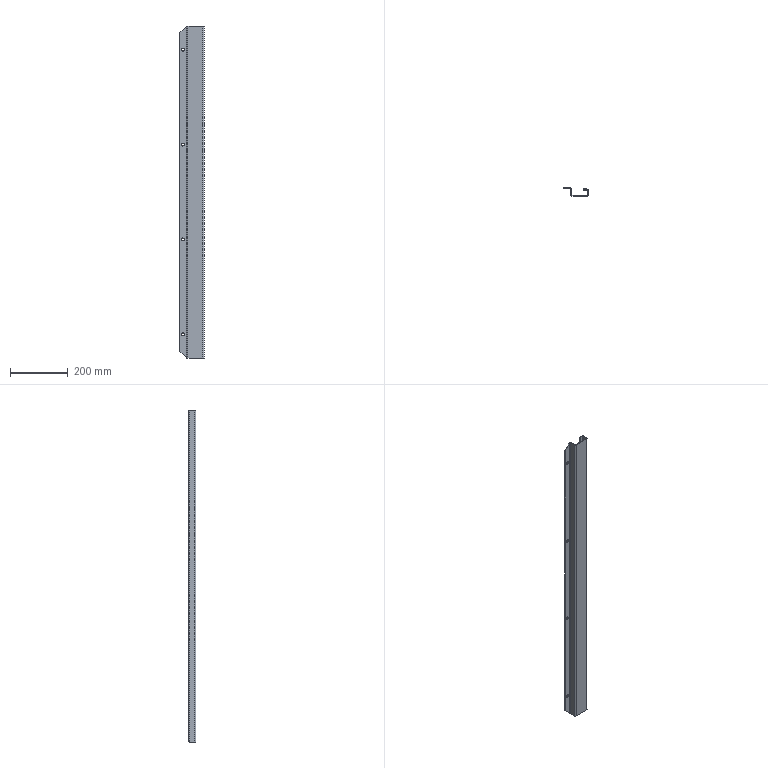Part | STEP file | 750038191 | 1 solid | 34 faces | box 84 x 27 x 1154 mm | volume 316306 mm3 | cylinder 16 | plane 16 | spline 2 | commonest cylinder face diameters 10.5 x8 4 x4 8 x4
STEP:
#1=CARTESIAN_POINT('',(-44.,27.,159.75));
#2=VERTEX_POINT('',#1);
#3=CARTESIAN_POINT('',(-44.,27.,170.25));
#4=VERTEX_POINT('',#3);
#5=CARTESIAN_POINT('',(-44.,27.,165.));
#6=DIRECTION('',(0.,1.,0.));
#7=DIRECTION('',(0.,0.,-1.));
#8=AXIS2_PLACEMENT_3D('',#5,#6,#7);
#9=CIRCLE('',#8,5.25);
#10=EDGE_CURVE('',#2,#4,#9,.T.);
#11=ORIENTED_EDGE('',*,*,#10,.T.);
#12=CARTESIAN_POINT('',(-44.,25.,170.25));
#13=VERTEX_POINT('',#12);
#14=CARTESIAN_POINT('',(-44.,1182.368,170.25));
#15=DIRECTION('',(0.,-1.,0.));
#16=VECTOR('',#15,1000.);
#17=LINE('',#14,#16);
#18=EDGE_CURVE('',#4,#13,#17,.T.);
#19=ORIENTED_EDGE('',*,*,#18,.T.);
#20=CARTESIAN_POINT('',(-44.,25.,159.75));
#21=VERTEX_POINT('',#20);
#22=CARTESIAN_POINT('',(-44.,25.,165.));
#23=DIRECTION('',(0.,1.,0.));
#24=DIRECTION('',(0.,0.,-1.));
#25=AXIS2_PLACEMENT_3D('',#22,#23,#24);
#26=CIRCLE('',#25,5.25);
#27=EDGE_CURVE('',#21,#13,#26,.T.);
#28=ORIENTED_EDGE('',*,*,#27,.F.);
#29=CARTESIAN_POINT('',(-44.,1182.368,159.75));
#30=DIRECTION('',(0.,-1.,0.));
#31=VECTOR('',#30,1000.);
#32=LINE('',#29,#31);
#33=EDGE_CURVE('',#2,#21,#32,.T.);
#34=ORIENTED_EDGE('',*,*,#33,.F.);
#35=EDGE_LOOP('',(#11,#19,#28,#34));
#36=FACE_OUTER_BOUND('',#35,.T.);
#37=CARTESIAN_POINT('',(-44.,1182.368,165.));
#38=DIRECTION('',(0.,-1.,0.));
#39=DIRECTION('',(0.,0.,-1.));
#40=AXIS2_PLACEMENT_3D('',#37,#38,#39);
#41=CYLINDRICAL_SURFACE('',#40,5.25);
#42=ADVANCED_FACE('',(#36),#41,.F.);
#43=CARTESIAN_POINT('',(-44.,27.,-500.25));
#44=VERTEX_POINT('',#43);
#45=CARTESIAN_POINT('',(-44.,27.,-489.75));
#46=VERTEX_POINT('',#45);
#47=CARTESIAN_POINT('',(-44.,27.,-495.));
#48=DIRECTION('',(0.,1.,0.));
#49=DIRECTION('',(0.,0.,-1.));
#50=AXIS2_PLACEMENT_3D('',#47,#48,#49);
#51=CIRCLE('',#50,5.25);
#52=EDGE_CURVE('',#44,#46,#51,.T.);
#53=ORIENTED_EDGE('',*,*,#52,.T.);
#54=CARTESIAN_POINT('',(-44.,25.,-489.75));
#55=VERTEX_POINT('',#54);
#56=CARTESIAN_POINT('',(-44.,1182.368,-489.75));
#57=DIRECTION('',(0.,-1.,0.));
#58=VECTOR('',#57,1000.);
#59=LINE('',#56,#58);
#60=EDGE_CURVE('',#46,#55,#59,.T.);
#61=ORIENTED_EDGE('',*,*,#60,.T.);
#62=CARTESIAN_POINT('',(-44.,25.,-500.25));
#63=VERTEX_POINT('',#62);
#64=CARTESIAN_POINT('',(-44.,25.,-495.));
#65=DIRECTION('',(0.,1.,0.));
#66=DIRECTION('',(0.,0.,-1.));
#67=AXIS2_PLACEMENT_3D('',#64,#65,#66);
#68=CIRCLE('',#67,5.25);
#69=EDGE_CURVE('',#63,#55,#68,.T.);
#70=ORIENTED_EDGE('',*,*,#69,.F.);
#71=CARTESIAN_POINT('',(-44.,1182.368,-500.25));
#72=DIRECTION('',(0.,-1.,0.));
#73=VECTOR('',#72,1000.);
#74=LINE('',#71,#73);
#75=EDGE_CURVE('',#44,#63,#74,.T.);
#76=ORIENTED_EDGE('',*,*,#75,.F.);
#77=EDGE_LOOP('',(#53,#61,#70,#76));
#78=FACE_OUTER_BOUND('',#77,.T.);
#79=CARTESIAN_POINT('',(-44.,1182.368,-495.));
#80=DIRECTION('',(0.,-1.,0.));
#81=DIRECTION('',(0.,0.,-1.));
#82=AXIS2_PLACEMENT_3D('',#79,#80,#81);
#83=CYLINDRICAL_SURFACE('',#82,5.25);
#84=ADVANCED_FACE('',(#78),#83,.F.);
#85=CARTESIAN_POINT('',(-44.,27.,-170.25));
#86=VERTEX_POINT('',#85);
#87=CARTESIAN_POINT('',(-44.,27.,-159.75));
#88=VERTEX_POINT('',#87);
#89=CARTESIAN_POINT('',(-44.,27.,-165.));
#90=DIRECTION('',(0.,1.,0.));
#91=DIRECTION('',(0.,0.,-1.));
#92=AXIS2_PLACEMENT_3D('',#89,#90,#91);
#93=CIRCLE('',#92,5.25);
#94=EDGE_CURVE('',#86,#88,#93,.T.);
#95=ORIENTED_EDGE('',*,*,#94,.T.);
#96=CARTESIAN_POINT('',(-44.,25.,-159.75));
#97=VERTEX_POINT('',#96);
#98=CARTESIAN_POINT('',(-44.,1182.368,-159.75));
#99=DIRECTION('',(0.,-1.,0.));
#100=VECTOR('',#99,1000.);
#101=LINE('',#98,#100);
#102=EDGE_CURVE('',#88,#97,#101,.T.);
#103=ORIENTED_EDGE('',*,*,#102,.T.);
#104=CARTESIAN_POINT('',(-44.,25.,-170.25));
#105=VERTEX_POINT('',#104);
#106=CARTESIAN_POINT('',(-44.,25.,-165.));
#107=DIRECTION('',(0.,1.,0.));
#108=DIRECTION('',(0.,0.,-1.));
#109=AXIS2_PLACEMENT_3D('',#106,#107,#108);
#110=CIRCLE('',#109,5.25);
#111=EDGE_CURVE('',#105,#97,#110,.T.);
#112=ORIENTED_EDGE('',*,*,#111,.F.);
#113=CARTESIAN_POINT('',(-44.,1182.368,-170.25));
#114=DIRECTION('',(0.,-1.,0.));
#115=VECTOR('',#114,1000.);
#116=LINE('',#113,#115);
#117=EDGE_CURVE('',#86,#105,#116,.T.);
#118=ORIENTED_EDGE('',*,*,#117,.F.);
#119=EDGE_LOOP('',(#95,#103,#112,#118));
#120=FACE_OUTER_BOUND('',#119,.T.);
#121=CARTESIAN_POINT('',(-44.,1182.368,-165.));
#122=DIRECTION('',(0.,-1.,0.));
#123=DIRECTION('',(0.,0.,-1.));
#124=AXIS2_PLACEMENT_3D('',#121,#122,#123);
#125=CYLINDRICAL_SURFACE('',#124,5.25);
#126=ADVANCED_FACE('',(#120),#125,.F.);
#127=CARTESIAN_POINT('',(-44.,27.,489.75));
#128=VERTEX_POINT('',#127);
#129=CARTESIAN_POINT('',(-44.,27.,500.25));
#130=VERTEX_POINT('',#129);
#131=CARTESIAN_POINT('',(-44.,27.,495.));
#132=DIRECTION('',(0.,1.,0.));
#133=DIRECTION('',(0.,0.,-1.));
#134=AXIS2_PLACEMENT_3D('',#131,#132,#133);
#135=CIRCLE('',#134,5.25);
#136=EDGE_CURVE('',#128,#130,#135,.T.);
#137=ORIENTED_EDGE('',*,*,#136,.T.);
#138=CARTESIAN_POINT('',(-44.,25.,500.25));
#139=VERTEX_POINT('',#138);
#140=CARTESIAN_POINT('',(-44.,1182.368,500.25));
#141=DIRECTION('',(0.,-1.,0.));
#142=VECTOR('',#141,1000.);
#143=LINE('',#140,#142);
#144=EDGE_CURVE('',#130,#139,#143,.T.);
#145=ORIENTED_EDGE('',*,*,#144,.T.);
#146=CARTESIAN_POINT('',(-44.,25.,489.75));
#147=VERTEX_POINT('',#146);
#148=CARTESIAN_POINT('',(-44.,25.,495.));
#149=DIRECTION('',(0.,1.,0.));
#150=DIRECTION('',(0.,0.,-1.));
#151=AXIS2_PLACEMENT_3D('',#148,#149,#150);
#152=CIRCLE('',#151,5.25);
#153=EDGE_CURVE('',#147,#139,#152,.T.);
#154=ORIENTED_EDGE('',*,*,#153,.F.);
#155=CARTESIAN_POINT('',(-44.,1182.368,489.75));
#156=DIRECTION('',(0.,-1.,0.));
#157=VECTOR('',#156,1000.);
#158=LINE('',#155,#157);
#159=EDGE_CURVE('',#128,#147,#158,.T.);
#160=ORIENTED_EDGE('',*,*,#159,.F.);
#161=EDGE_LOOP('',(#137,#145,#154,#160));
#162=FACE_OUTER_BOUND('',#161,.T.);
#163=CARTESIAN_POINT('',(-44.,1182.368,495.));
#164=DIRECTION('',(0.,-1.,0.));
#165=DIRECTION('',(0.,0.,-1.));
#166=AXIS2_PLACEMENT_3D('',#163,#164,#165);
#167=CYLINDRICAL_SURFACE('',#166,5.25);
#168=ADVANCED_FACE('',(#162),#167,.F.);
#169=CARTESIAN_POINT('',(26.,0.,577.));
#170=VERTEX_POINT('',#169);
#171=CARTESIAN_POINT('',(-26.,0.,577.));
#172=VERTEX_POINT('',#171);
#173=CARTESIAN_POINT('',(30.,0.,577.));
#174=DIRECTION('',(-1.,0.,0.));
#175=VECTOR('',#174,1000.);
#176=LINE('',#173,#175);
#177=EDGE_CURVE('',#170,#172,#176,.T.);
#178=ORIENTED_EDGE('',*,*,#177,.T.);
#179=CARTESIAN_POINT('',(-26.,0.,-577.));
#180=VERTEX_POINT('',#179);
#181=CARTESIAN_POINT('',(-26.,0.,577.));
#182=DIRECTION('',(0.,0.,-1.));
#183=VECTOR('',#182,1000.);
#184=LINE('',#181,#183);
#185=EDGE_CURVE('',#172,#180,#184,.T.);
#186=ORIENTED_EDGE('',*,*,#185,.T.);
#187=CARTESIAN_POINT('',(26.,0.,-577.));
#188=VERTEX_POINT('',#187);
#189=CARTESIAN_POINT('',(30.,0.,-577.));
#190=DIRECTION('',(1.,0.,0.));
#191=VECTOR('',#190,1000.);
#192=LINE('',#189,#191);
#193=EDGE_CURVE('',#180,#188,#192,.T.);
#194=ORIENTED_EDGE('',*,*,#193,.T.);
#195=CARTESIAN_POINT('',(26.,0.,577.));
#196=DIRECTION('',(0.,0.,1.));
#197=VECTOR('',#196,1000.);
#198=LINE('',#195,#197);
#199=EDGE_CURVE('',#188,#170,#198,.T.);
#200=ORIENTED_EDGE('',*,*,#199,.T.);
#201=EDGE_LOOP('',(#178,#186,#194,#200));
#202=FACE_OUTER_BOUND('',#201,.T.);
#203=CARTESIAN_POINT('',(30.,0.,577.));
#204=DIRECTION('',(0.,-1.,0.));
#205=DIRECTION('',(1.,0.,0.));
#206=AXIS2_PLACEMENT_3D('',#203,#204,#205);
#207=PLANE('',#206);
#208=ADVANCED_FACE('',(#202),#207,.T.);
#209=CARTESIAN_POINT('',(-30.,4.,577.));
#210=VERTEX_POINT('',#209);
#211=CARTESIAN_POINT('',(-26.,4.,577.));
#212=DIRECTION('',(0.,0.,-1.));
#213=DIRECTION('',(-1.,0.,0.));
#214=AXIS2_PLACEMENT_3D('',#211,#212,#213);
#215=CIRCLE('',#214,4.);
#216=EDGE_CURVE('',#172,#210,#215,.T.);
#217=ORIENTED_EDGE('',*,*,#216,.T.);
#218=CARTESIAN_POINT('',(-30.,4.,-577.));
#219=VERTEX_POINT('',#218);
#220=CARTESIAN_POINT('',(-30.,4.,577.));
#221=DIRECTION('',(0.,0.,-1.));
#222=VECTOR('',#221,1000.);
#223=LINE('',#220,#222);
#224=EDGE_CURVE('',#210,#219,#223,.T.);
#225=ORIENTED_EDGE('',*,*,#224,.T.);
#226=CARTESIAN_POINT('',(-26.,4.,-577.));
#227=DIRECTION('',(0.,0.,1.));
#228=DIRECTION('',(-1.,0.,0.));
#229=AXIS2_PLACEMENT_3D('',#226,#227,#228);
#230=CIRCLE('',#229,4.);
#231=EDGE_CURVE('',#219,#180,#230,.T.);
#232=ORIENTED_EDGE('',*,*,#231,.T.);
#233=ORIENTED_EDGE('',*,*,#185,.F.);
#234=EDGE_LOOP('',(#217,#225,#232,#233));
#235=FACE_OUTER_BOUND('',#234,.T.);
#236=CARTESIAN_POINT('',(-26.,4.,577.));
#237=DIRECTION('',(0.,0.,-1.));
#238=DIRECTION('',(-1.,0.,0.));
#239=AXIS2_PLACEMENT_3D('',#236,#237,#238);
#240=CYLINDRICAL_SURFACE('',#239,4.);
#241=ADVANCED_FACE('',(#235),#240,.T.);
#242=CARTESIAN_POINT('',(26.,2.,577.));
#243=VERTEX_POINT('',#242);
#244=CARTESIAN_POINT('',(-26.,2.,577.));
#245=VERTEX_POINT('',#244);
#246=CARTESIAN_POINT('',(-30.,2.,577.));
#247=DIRECTION('',(-1.,0.,0.));
#248=VECTOR('',#247,1000.);
#249=LINE('',#246,#248);
#250=EDGE_CURVE('',#243,#245,#249,.T.);
#251=ORIENTED_EDGE('',*,*,#250,.T.);
#252=CARTESIAN_POINT('',(-28.,4.,577.));
#253=VERTEX_POINT('',#252);
#254=CARTESIAN_POINT('',(-26.,4.,577.));
#255=DIRECTION('',(0.,0.,-1.));
#256=DIRECTION('',(-1.,0.,0.));
#257=AXIS2_PLACEMENT_3D('',#254,#255,#256);
#258=CIRCLE('',#257,2.);
#259=EDGE_CURVE('',#245,#253,#258,.T.);
#260=ORIENTED_EDGE('',*,*,#259,.T.);
#261=CARTESIAN_POINT('',(-28.,23.,577.));
#262=VERTEX_POINT('',#261);
#263=CARTESIAN_POINT('',(-28.,25.,577.));
#264=DIRECTION('',(0.,1.,0.));
#265=VECTOR('',#264,1000.);
#266=LINE('',#263,#265);
#267=EDGE_CURVE('',#253,#262,#266,.T.);
#268=ORIENTED_EDGE('',*,*,#267,.T.);
#269=CARTESIAN_POINT('',(-30.,23.,577.));
#270=VERTEX_POINT('',#269);
#271=CARTESIAN_POINT('',(-30.,23.,577.));
#272=DIRECTION('',(-1.,0.,0.));
#273=VECTOR('',#272,1000.);
#274=LINE('',#271,#273);
#275=EDGE_CURVE('',#262,#270,#274,.T.);
#276=ORIENTED_EDGE('',*,*,#275,.T.);
#277=CARTESIAN_POINT('',(-30.,25.,577.));
#278=DIRECTION('',(0.,-1.,0.));
#279=VECTOR('',#278,1000.);
#280=LINE('',#277,#279);
#281=EDGE_CURVE('',#270,#210,#280,.T.);
#282=ORIENTED_EDGE('',*,*,#281,.T.);
#283=ORIENTED_EDGE('',*,*,#216,.F.);
#284=ORIENTED_EDGE('',*,*,#177,.F.);
#285=CARTESIAN_POINT('',(30.,4.,577.));
#286=VERTEX_POINT('',#285);
#287=CARTESIAN_POINT('',(26.,4.,577.));
#288=DIRECTION('',(0.,0.,1.));
#289=DIRECTION('',(-1.,0.,0.));
#290=AXIS2_PLACEMENT_3D('',#287,#288,#289);
#291=CIRCLE('',#290,4.);
#292=EDGE_CURVE('',#170,#286,#291,.T.);
#293=ORIENTED_EDGE('',*,*,#292,.T.);
#294=CARTESIAN_POINT('',(30.,19.,577.));
#295=VERTEX_POINT('',#294);
#296=CARTESIAN_POINT('',(30.,25.,577.));
#297=DIRECTION('',(0.,1.,0.));
#298=VECTOR('',#297,1000.);
#299=LINE('',#296,#298);
#300=EDGE_CURVE('',#286,#295,#299,.T.);
#301=ORIENTED_EDGE('',*,*,#300,.T.);
#302=CARTESIAN_POINT('',(26.,23.,577.));
#303=VERTEX_POINT('',#302);
#304=CARTESIAN_POINT('',(26.,19.,577.));
#305=DIRECTION('',(0.,0.,1.));
#306=DIRECTION('',(-1.,0.,0.));
#307=AXIS2_PLACEMENT_3D('',#304,#305,#306);
#308=CIRCLE('',#307,4.);
#309=EDGE_CURVE('',#295,#303,#308,.T.);
#310=ORIENTED_EDGE('',*,*,#309,.T.);
#311=CARTESIAN_POINT('',(15.,23.,577.));
#312=VERTEX_POINT('',#311);
#313=CARTESIAN_POINT('',(-30.,23.,577.));
#314=DIRECTION('',(-1.,0.,0.));
#315=VECTOR('',#314,1000.);
#316=LINE('',#313,#315);
#317=EDGE_CURVE('',#303,#312,#316,.T.);
#318=ORIENTED_EDGE('',*,*,#317,.T.);
#319=CARTESIAN_POINT('',(15.,21.,577.));
#320=VERTEX_POINT('',#319);
#321=CARTESIAN_POINT('',(15.,25.,577.));
#322=DIRECTION('',(0.,-1.,0.));
#323=VECTOR('',#322,1000.);
#324=LINE('',#321,#323);
#325=EDGE_CURVE('',#312,#320,#324,.T.);
#326=ORIENTED_EDGE('',*,*,#325,.T.);
#327=CARTESIAN_POINT('',(26.,21.,577.));
#328=VERTEX_POINT('',#327);
#329=CARTESIAN_POINT('',(-30.,21.,577.));
#330=DIRECTION('',(1.,0.,0.));
#331=VECTOR('',#330,1000.);
#332=LINE('',#329,#331);
#333=EDGE_CURVE('',#320,#328,#332,.T.);
#334=ORIENTED_EDGE('',*,*,#333,.T.);
#335=CARTESIAN_POINT('',(28.,19.,577.));
#336=VERTEX_POINT('',#335);
#337=CARTESIAN_POINT('',(26.,19.,577.));
#338=DIRECTION('',(0.,0.,-1.));
#339=DIRECTION('',(-1.,0.,0.));
#340=AXIS2_PLACEMENT_3D('',#337,#338,#339);
#341=CIRCLE('',#340,2.);
#342=EDGE_CURVE('',#328,#336,#341,.T.);
#343=ORIENTED_EDGE('',*,*,#342,.T.);
#344=CARTESIAN_POINT('',(28.,4.,577.));
#345=VERTEX_POINT('',#344);
#346=CARTESIAN_POINT('',(28.,25.,577.));
#347=DIRECTION('',(0.,-1.,0.));
#348=VECTOR('',#347,1000.);
#349=LINE('',#346,#348);
#350=EDGE_CURVE('',#336,#345,#349,.T.);
#351=ORIENTED_EDGE('',*,*,#350,.T.);
#352=CARTESIAN_POINT('',(26.,4.,577.));
#353=DIRECTION('',(0.,0.,-1.));
#354=DIRECTION('',(-1.,0.,0.));
#355=AXIS2_PLACEMENT_3D('',#352,#353,#354);
#356=CIRCLE('',#355,2.);
#357=EDGE_CURVE('',#345,#243,#356,.T.);
#358=ORIENTED_EDGE('',*,*,#357,.T.);
#359=EDGE_LOOP('',(#251,#260,#268,#276,#282,#283,#284,#293,#301,#310,#318,#326,#334,#343,#351,#358));
#360=FACE_OUTER_BOUND('',#359,.T.);
#361=CARTESIAN_POINT('',(-30.,25.,577.));
#362=DIRECTION('',(0.,0.,1.));
#363=DIRECTION('',(1.,0.,0.));
#364=AXIS2_PLACEMENT_3D('',#361,#362,#363);
#365=PLANE('',#364);
#366=ADVANCED_FACE('',(#360),#365,.T.);
#367=ORIENTED_EDGE('',*,*,#292,.F.);
#368=ORIENTED_EDGE('',*,*,#199,.F.);
#369=CARTESIAN_POINT('',(30.,4.,-577.));
#370=VERTEX_POINT('',#369);
#371=CARTESIAN_POINT('',(26.,4.,-577.));
#372=DIRECTION('',(0.,0.,1.));
#373=DIRECTION('',(-1.,0.,0.));
#374=AXIS2_PLACEMENT_3D('',#371,#372,#373);
#375=CIRCLE('',#374,4.);
#376=EDGE_CURVE('',#188,#370,#375,.T.);
#377=ORIENTED_EDGE('',*,*,#376,.T.);
#378=CARTESIAN_POINT('',(30.,4.,577.));
#379=DIRECTION('',(0.,0.,1.));
#380=VECTOR('',#379,1000.);
#381=LINE('',#378,#380);
#382=EDGE_CURVE('',#370,#286,#381,.T.);
#383=ORIENTED_EDGE('',*,*,#382,.T.);
#384=EDGE_LOOP('',(#367,#368,#377,#383));
#385=FACE_OUTER_BOUND('',#384,.T.);
#386=CARTESIAN_POINT('',(26.,4.,577.));
#387=DIRECTION('',(0.,0.,-1.));
#388=DIRECTION('',(-1.,0.,0.));
#389=AXIS2_PLACEMENT_3D('',#386,#387,#388);
#390=CYLINDRICAL_SURFACE('',#389,4.);
#391=ADVANCED_FACE('',(#385),#390,.T.);
#392=CARTESIAN_POINT('',(-28.,4.,-577.));
#393=VERTEX_POINT('',#392);
#394=CARTESIAN_POINT('',(-28.,23.,-577.));
#395=VERTEX_POINT('',#394);
#396=CARTESIAN_POINT('',(-28.,23.,-577.));
#397=DIRECTION('',(0.,1.,0.));
#398=VECTOR('',#397,1000.);
#399=LINE('',#396,#398);
#400=EDGE_CURVE('',#393,#395,#399,.T.);
#401=ORIENTED_EDGE('',*,*,#400,.F.);
#402=CARTESIAN_POINT('',(-26.,2.,-577.));
#403=VERTEX_POINT('',#402);
#404=CARTESIAN_POINT('',(-26.,4.,-577.));
#405=DIRECTION('',(0.,0.,-1.));
#406=DIRECTION('',(-1.,0.,0.));
#407=AXIS2_PLACEMENT_3D('',#404,#405,#406);
#408=CIRCLE('',#407,2.);
#409=EDGE_CURVE('',#403,#393,#408,.T.);
#410=ORIENTED_EDGE('',*,*,#409,.F.);
#411=CARTESIAN_POINT('',(26.,2.,-577.));
#412=VERTEX_POINT('',#411);
#413=CARTESIAN_POINT('',(15.,2.,-577.));
#414=DIRECTION('',(-1.,0.,0.));
#415=VECTOR('',#414,1000.);
#416=LINE('',#413,#415);
#417=EDGE_CURVE('',#412,#403,#416,.T.);
#418=ORIENTED_EDGE('',*,*,#417,.F.);
#419=CARTESIAN_POINT('',(28.,4.,-577.));
#420=VERTEX_POINT('',#419);
#421=CARTESIAN_POINT('',(26.,4.,-577.));
#422=DIRECTION('',(0.,0.,-1.));
#423=DIRECTION('',(-1.,0.,0.));
#424=AXIS2_PLACEMENT_3D('',#421,#422,#423);
#425=CIRCLE('',#424,2.);
#426=EDGE_CURVE('',#420,#412,#425,.T.);
#427=ORIENTED_EDGE('',*,*,#426,.F.);
#428=CARTESIAN_POINT('',(28.,19.,-577.));
#429=VERTEX_POINT('',#428);
#430=CARTESIAN_POINT('',(28.,23.,-577.));
#431=DIRECTION('',(0.,-1.,0.));
#432=VECTOR('',#431,1000.);
#433=LINE('',#430,#432);
#434=EDGE_CURVE('',#429,#420,#433,.T.);
#435=ORIENTED_EDGE('',*,*,#434,.F.);
#436=CARTESIAN_POINT('',(26.,21.,-577.));
#437=VERTEX_POINT('',#436);
#438=CARTESIAN_POINT('',(26.,19.,-577.));
#439=DIRECTION('',(0.,0.,-1.));
#440=DIRECTION('',(-1.,0.,0.));
#441=AXIS2_PLACEMENT_3D('',#438,#439,#440);
#442=CIRCLE('',#441,2.);
#443=EDGE_CURVE('',#437,#429,#442,.T.);
#444=ORIENTED_EDGE('',*,*,#443,.F.);
#445=CARTESIAN_POINT('',(15.,21.,-577.));
#446=VERTEX_POINT('',#445);
#447=CARTESIAN_POINT('',(15.,21.,-577.));
#448=DIRECTION('',(1.,0.,0.));
#449=VECTOR('',#448,1000.);
#450=LINE('',#447,#449);
#451=EDGE_CURVE('',#446,#437,#450,.T.);
#452=ORIENTED_EDGE('',*,*,#451,.F.);
#453=CARTESIAN_POINT('',(15.,23.,-577.));
#454=VERTEX_POINT('',#453);
#455=CARTESIAN_POINT('',(15.,23.,-577.));
#456=DIRECTION('',(0.,-1.,0.));
#457=VECTOR('',#456,1000.);
#458=LINE('',#455,#457);
#459=EDGE_CURVE('',#454,#446,#458,.T.);
#460=ORIENTED_EDGE('',*,*,#459,.F.);
#461=CARTESIAN_POINT('',(26.,23.,-577.));
#462=VERTEX_POINT('',#461);
#463=CARTESIAN_POINT('',(15.,23.,-577.));
#464=DIRECTION('',(-1.,0.,0.));
#465=VECTOR('',#464,1000.);
#466=LINE('',#463,#465);
#467=EDGE_CURVE('',#462,#454,#466,.T.);
#468=ORIENTED_EDGE('',*,*,#467,.F.);
#469=CARTESIAN_POINT('',(30.,19.,-577.));
#470=VERTEX_POINT('',#469);
#471=CARTESIAN_POINT('',(26.,19.,-577.));
#472=DIRECTION('',(0.,0.,1.));
#473=DIRECTION('',(-1.,0.,0.));
#474=AXIS2_PLACEMENT_3D('',#471,#472,#473);
#475=CIRCLE('',#474,4.);
#476=EDGE_CURVE('',#470,#462,#475,.T.);
#477=ORIENTED_EDGE('',*,*,#476,.F.);
#478=CARTESIAN_POINT('',(30.,23.,-577.));
#479=DIRECTION('',(0.,1.,0.));
#480=VECTOR('',#479,1000.);
#481=LINE('',#478,#480);
#482=EDGE_CURVE('',#370,#470,#481,.T.);
#483=ORIENTED_EDGE('',*,*,#482,.F.);
#484=ORIENTED_EDGE('',*,*,#376,.F.);
#485=ORIENTED_EDGE('',*,*,#193,.F.);
#486=ORIENTED_EDGE('',*,*,#231,.F.);
#487=CARTESIAN_POINT('',(-30.,23.,-577.));
#488=VERTEX_POINT('',#487);
#489=CARTESIAN_POINT('',(-30.,23.,-577.));
#490=DIRECTION('',(0.,-1.,0.));
#491=VECTOR('',#490,1000.);
#492=LINE('',#489,#491);
#493=EDGE_CURVE('',#488,#219,#492,.T.);
#494=ORIENTED_EDGE('',*,*,#493,.F.);
#495=CARTESIAN_POINT('',(15.,23.,-577.));
#496=DIRECTION('',(-1.,0.,0.));
#497=VECTOR('',#496,1000.);
#498=LINE('',#495,#497);
#499=EDGE_CURVE('',#395,#488,#498,.T.);
#500=ORIENTED_EDGE('',*,*,#499,.F.);
#501=EDGE_LOOP('',(#401,#410,#418,#427,#435,#444,#452,#460,#468,#477,#483,#484,#485,#486,#494,#500));
#502=FACE_OUTER_BOUND('',#501,.T.);
#503=CARTESIAN_POINT('',(15.,23.,-577.));
#504=DIRECTION('',(0.,0.,1.));
#505=DIRECTION('',(1.,0.,0.));
#506=AXIS2_PLACEMENT_3D('',#503,#504,#505);
#507=PLANE('',#506);
#508=ADVANCED_FACE('',(#502),#507,.F.);
#509=ORIENTED_EDGE('',*,*,#281,.F.);
#510=CARTESIAN_POINT('',(-30.,23.,577.));
#511=DIRECTION('',(0.,0.,-1.));
#512=VECTOR('',#511,1000.);
#513=LINE('',#510,#512);
#514=EDGE_CURVE('',#270,#488,#513,.T.);
#515=ORIENTED_EDGE('',*,*,#514,.T.);
#516=ORIENTED_EDGE('',*,*,#493,.T.);
#517=ORIENTED_EDGE('',*,*,#224,.F.);
#518=EDGE_LOOP('',(#509,#515,#516,#517));
#519=FACE_OUTER_BOUND('',#518,.T.);
#520=CARTESIAN_POINT('',(-30.,0.,577.));
#521=DIRECTION('',(-1.,0.,0.));
#522=DIRECTION('',(0.,-1.,0.));
#523=AXIS2_PLACEMENT_3D('',#520,#521,#522);
#524=PLANE('',#523);
#525=ADVANCED_FACE('',(#519),#524,.T.);
#526=CARTESIAN_POINT('',(-28.,4.,577.));
#527=DIRECTION('',(0.,0.,-1.));
#528=VECTOR('',#527,1000.);
#529=LINE('',#526,#528);
#530=EDGE_CURVE('',#253,#393,#529,.T.);
#531=ORIENTED_EDGE('',*,*,#530,.F.);
#532=ORIENTED_EDGE('',*,*,#259,.F.);
#533=CARTESIAN_POINT('',(-26.,2.,577.));
#534=DIRECTION('',(0.,0.,1.));
#535=VECTOR('',#534,1000.);
#536=LINE('',#533,#535);
#537=EDGE_CURVE('',#403,#245,#536,.T.);
#538=ORIENTED_EDGE('',*,*,#537,.F.);
#539=ORIENTED_EDGE('',*,*,#409,.T.);
#540=EDGE_LOOP('',(#531,#532,#538,#539));
#541=FACE_OUTER_BOUND('',#540,.T.);
#542=CARTESIAN_POINT('',(-26.,4.,577.));
#543=DIRECTION('',(0.,0.,-1.));
#544=DIRECTION('',(-1.,0.,0.));
#545=AXIS2_PLACEMENT_3D('',#542,#543,#544);
#546=CYLINDRICAL_SURFACE('',#545,2.);
#547=ADVANCED_FACE('',(#541),#546,.F.);
#548=ORIENTED_EDGE('',*,*,#537,.T.);
#549=ORIENTED_EDGE('',*,*,#250,.F.);
#550=CARTESIAN_POINT('',(26.,2.,577.));
#551=DIRECTION('',(0.,0.,1.));
#552=VECTOR('',#551,1000.);
#553=LINE('',#550,#552);
#554=EDGE_CURVE('',#412,#243,#553,.T.);
#555=ORIENTED_EDGE('',*,*,#554,.F.);
#556=ORIENTED_EDGE('',*,*,#417,.T.);
#557=EDGE_LOOP('',(#548,#549,#555,#556));
#558=FACE_OUTER_BOUND('',#557,.T.);
#559=CARTESIAN_POINT('',(30.,2.,577.));
#560=DIRECTION('',(0.,-1.,0.));
#561=DIRECTION('',(1.,0.,0.));
#562=AXIS2_PLACEMENT_3D('',#559,#560,#561);
#563=PLANE('',#562);
#564=ADVANCED_FACE('',(#558),#563,.F.);
#565=ORIENTED_EDGE('',*,*,#554,.T.);
#566=ORIENTED_EDGE('',*,*,#357,.F.);
#567=CARTESIAN_POINT('',(28.,4.,577.));
#568=DIRECTION('',(0.,0.,1.));
#569=VECTOR('',#568,1000.);
#570=LINE('',#567,#569);
#571=EDGE_CURVE('',#420,#345,#570,.T.);
#572=ORIENTED_EDGE('',*,*,#571,.F.);
#573=ORIENTED_EDGE('',*,*,#426,.T.);
#574=EDGE_LOOP('',(#565,#566,#572,#573));
#575=FACE_OUTER_BOUND('',#574,.T.);
#576=CARTESIAN_POINT('',(26.,4.,577.));
#577=DIRECTION('',(0.,0.,-1.));
#578=DIRECTION('',(-1.,0.,0.));
#579=AXIS2_PLACEMENT_3D('',#576,#577,#578);
#580=CYLINDRICAL_SURFACE('',#579,2.);
#581=ADVANCED_FACE('',(#575),#580,.F.);
#582=ORIENTED_EDGE('',*,*,#571,.T.);
#583=ORIENTED_EDGE('',*,*,#350,.F.);
#584=CARTESIAN_POINT('',(28.,19.,577.));
#585=DIRECTION('',(0.,0.,1.));
#586=VECTOR('',#585,1000.);
#587=LINE('',#584,#586);
#588=EDGE_CURVE('',#429,#336,#587,.T.);
#589=ORIENTED_EDGE('',*,*,#588,.F.);
#590=ORIENTED_EDGE('',*,*,#434,.T.);
#591=EDGE_LOOP('',(#582,#583,#589,#590));
#592=FACE_OUTER_BOUND('',#591,.T.);
#593=CARTESIAN_POINT('',(28.,23.,577.));
#594=DIRECTION('',(1.,0.,0.));
#595=DIRECTION('',(0.,1.,0.));
#596=AXIS2_PLACEMENT_3D('',#593,#594,#595);
#597=PLANE('',#596);
#598=ADVANCED_FACE('',(#592),#597,.F.);
#599=ORIENTED_EDGE('',*,*,#588,.T.);
#600=ORIENTED_EDGE('',*,*,#342,.F.);
#601=CARTESIAN_POINT('',(26.,21.,577.));
#602=DIRECTION('',(0.,0.,1.));
#603=VECTOR('',#602,1000.);
#604=LINE('',#601,#603);
#605=EDGE_CURVE('',#437,#328,#604,.T.);
#606=ORIENTED_EDGE('',*,*,#605,.F.);
#607=ORIENTED_EDGE('',*,*,#443,.T.);
#608=EDGE_LOOP('',(#599,#600,#606,#607));
#609=FACE_OUTER_BOUND('',#608,.T.);
#610=CARTESIAN_POINT('',(26.,19.,577.));
#611=DIRECTION('',(0.,0.,-1.));
#612=DIRECTION('',(-1.,0.,0.));
#613=AXIS2_PLACEMENT_3D('',#610,#611,#612);
#614=CYLINDRICAL_SURFACE('',#613,2.);
#615=ADVANCED_FACE('',(#609),#614,.F.);
#616=ORIENTED_EDGE('',*,*,#605,.T.);
#617=ORIENTED_EDGE('',*,*,#333,.F.);
#618=CARTESIAN_POINT('',(15.,21.,577.));
#619=DIRECTION('',(0.,0.,1.));
#620=VECTOR('',#619,1000.);
#621=LINE('',#618,#620);
#622=EDGE_CURVE('',#446,#320,#621,.T.);
#623=ORIENTED_EDGE('',*,*,#622,.F.);
#624=ORIENTED_EDGE('',*,*,#451,.T.);
#625=EDGE_LOOP('',(#616,#617,#623,#624));
#626=FACE_OUTER_BOUND('',#625,.T.);
#627=CARTESIAN_POINT('',(15.,21.,577.));
#628=DIRECTION('',(0.,1.,0.));
#629=DIRECTION('',(0.,0.,1.));
#630=AXIS2_PLACEMENT_3D('',#627,#628,#629);
#631=PLANE('',#630);
#632=ADVANCED_FACE('',(#626),#631,.F.);
#633=ORIENTED_EDGE('',*,*,#325,.F.);
#634=CARTESIAN_POINT('',(15.,23.,577.));
#635=DIRECTION('',(0.,0.,1.));
#636=VECTOR('',#635,1000.);
#637=LINE('',#634,#636);
#638=EDGE_CURVE('',#454,#312,#637,.T.);
#639=ORIENTED_EDGE('',*,*,#638,.F.);
#640=ORIENTED_EDGE('',*,*,#459,.T.);
#641=ORIENTED_EDGE('',*,*,#622,.T.);
#642=EDGE_LOOP('',(#633,#639,#640,#641));
#643=FACE_OUTER_BOUND('',#642,.T.);
#644=CARTESIAN_POINT('',(15.,23.,577.));
#645=DIRECTION('',(1.,0.,0.));
#646=DIRECTION('',(0.,0.,-1.));
#647=AXIS2_PLACEMENT_3D('',#644,#645,#646);
#648=PLANE('',#647);
#649=ADVANCED_FACE('',(#643),#648,.F.);
#650=ORIENTED_EDGE('',*,*,#317,.F.);
#651=CARTESIAN_POINT('',(26.,23.,577.));
#652=DIRECTION('',(0.,0.,-1.));
#653=VECTOR('',#652,1000.);
#654=LINE('',#651,#653);
#655=EDGE_CURVE('',#303,#462,#654,.T.);
#656=ORIENTED_EDGE('',*,*,#655,.T.);
#657=ORIENTED_EDGE('',*,*,#467,.T.);
#658=ORIENTED_EDGE('',*,*,#638,.T.);
#659=EDGE_LOOP('',(#650,#656,#657,#658));
#660=FACE_OUTER_BOUND('',#659,.T.);
#661=CARTESIAN_POINT('',(15.,23.,577.));
#662=DIRECTION('',(0.,1.,0.));
#663=DIRECTION('',(0.,0.,1.));
#664=AXIS2_PLACEMENT_3D('',#661,#662,#663);
#665=PLANE('',#664);
#666=ADVANCED_FACE('',(#660),#665,.T.);
#667=ORIENTED_EDGE('',*,*,#309,.F.);
#668=CARTESIAN_POINT('',(30.,19.,577.));
#669=DIRECTION('',(0.,0.,-1.));
#670=VECTOR('',#669,1000.);
#671=LINE('',#668,#670);
#672=EDGE_CURVE('',#295,#470,#671,.T.);
#673=ORIENTED_EDGE('',*,*,#672,.T.);
#674=ORIENTED_EDGE('',*,*,#476,.T.);
#675=ORIENTED_EDGE('',*,*,#655,.F.);
#676=EDGE_LOOP('',(#667,#673,#674,#675));
#677=FACE_OUTER_BOUND('',#676,.T.);
#678=CARTESIAN_POINT('',(26.,19.,577.));
#679=DIRECTION('',(0.,0.,-1.));
#680=DIRECTION('',(-1.,0.,0.));
#681=AXIS2_PLACEMENT_3D('',#678,#679,#680);
#682=CYLINDRICAL_SURFACE('',#681,4.);
#683=ADVANCED_FACE('',(#677),#682,.T.);
#684=ORIENTED_EDGE('',*,*,#300,.F.);
#685=ORIENTED_EDGE('',*,*,#382,.F.);
#686=ORIENTED_EDGE('',*,*,#482,.T.);
#687=ORIENTED_EDGE('',*,*,#672,.F.);
#688=EDGE_LOOP('',(#684,#685,#686,#687));
#689=FACE_OUTER_BOUND('',#688,.T.);
#690=CARTESIAN_POINT('',(30.,23.,577.));
#691=DIRECTION('',(1.,0.,0.));
#692=DIRECTION('',(0.,1.,0.));
#693=AXIS2_PLACEMENT_3D('',#690,#691,#692);
#694=PLANE('',#693);
#695=ADVANCED_FACE('',(#689),#694,.T.);
#696=ORIENTED_EDGE('',*,*,#275,.F.);
#697=CARTESIAN_POINT('',(-32.,27.,575.));
#698=VERTEX_POINT('',#697);
#699=CARTESIAN_POINT('',(-28.,23.,577.));
#700=CARTESIAN_POINT('',(-28.,25.,577.));
#701=CARTESIAN_POINT('',(-29.333,27.,576.333));
#702=CARTESIAN_POINT('',(-32.,27.,575.));
#703=(BOUNDED_CURVE()B_SPLINE_CURVE(3,(#699,#700,#701,#702),.UNSPECIFIED.,.F.,.T.)B_SPLINE_CURVE_WITH_KNOTS((4,4),(0.,0.006653),.UNSPECIFIED.)CURVE()GEOMETRIC_REPRESENTATION_ITEM()RATIONAL_B_SPLINE_CURVE((1.,0.6667,0.5,0.5))REPRESENTATION_ITEM(''));
#704=EDGE_CURVE('',#262,#698,#703,.T.);
#705=ORIENTED_EDGE('',*,*,#704,.T.);
#706=CARTESIAN_POINT('',(-32.,25.,575.));
#707=VERTEX_POINT('',#706);
#708=CARTESIAN_POINT('',(-32.,26.,575.));
#709=DIRECTION('',(0.,-1.,0.));
#710=VECTOR('',#709,1000.);
#711=LINE('',#708,#710);
#712=EDGE_CURVE('',#698,#707,#711,.T.);
#713=ORIENTED_EDGE('',*,*,#712,.T.);
#714=CARTESIAN_POINT('',(-32.,25.,575.));
#715=CARTESIAN_POINT('',(-30.667,25.,576.333));
#716=CARTESIAN_POINT('',(-30.,24.,577.));
#717=CARTESIAN_POINT('',(-30.,23.,577.));
#718=(BOUNDED_CURVE()B_SPLINE_CURVE(3,(#714,#715,#716,#717),.UNSPECIFIED.,.F.,.F.)B_SPLINE_CURVE_WITH_KNOTS((4,4),(0.,0.003785),.UNSPECIFIED.)CURVE()GEOMETRIC_REPRESENTATION_ITEM()RATIONAL_B_SPLINE_CURVE((0.5,0.5,0.6667,1.))REPRESENTATION_ITEM(''));
#719=EDGE_CURVE('',#707,#270,#718,.T.);
#720=ORIENTED_EDGE('',*,*,#719,.T.);
#721=EDGE_LOOP('',(#696,#705,#713,#720));
#722=FACE_OUTER_BOUND('',#721,.T.);
#723=CARTESIAN_POINT('',(-34.,23.,573.));
#724=CARTESIAN_POINT('',(-34.667,23.,573.));
#725=CARTESIAN_POINT('',(-35.333,23.,573.));
#726=CARTESIAN_POINT('',(-36.,23.,573.));
#727=CARTESIAN_POINT('',(-34.,27.,573.));
#728=CARTESIAN_POINT('',(-34.667,28.333,573.));
#729=CARTESIAN_POINT('',(-35.333,29.667,573.));
#730=CARTESIAN_POINT('',(-36.,31.,573.));
#731=CARTESIAN_POINT('',(-30.,27.,577.));
#732=CARTESIAN_POINT('',(-29.333,28.333,577.));
#733=CARTESIAN_POINT('',(-28.667,29.667,577.));
#734=CARTESIAN_POINT('',(-28.,31.,577.));
#735=CARTESIAN_POINT('',(-30.,23.,577.));
#736=CARTESIAN_POINT('',(-29.333,23.,577.));
#737=CARTESIAN_POINT('',(-28.667,23.,577.));
#738=CARTESIAN_POINT('',(-28.,23.,577.));
#739=CARTESIAN_POINT('',(-30.,19.,577.));
#740=CARTESIAN_POINT('',(-29.333,17.667,577.));
#741=CARTESIAN_POINT('',(-28.667,16.333,577.));
#742=CARTESIAN_POINT('',(-28.,15.,577.));
#743=CARTESIAN_POINT('',(-34.,19.,573.));
#744=CARTESIAN_POINT('',(-34.667,17.667,573.));
#745=CARTESIAN_POINT('',(-35.333,16.333,573.));
#746=CARTESIAN_POINT('',(-36.,15.,573.));
#747=CARTESIAN_POINT('',(-34.,23.,573.));
#748=CARTESIAN_POINT('',(-34.667,23.,573.));
#749=CARTESIAN_POINT('',(-35.333,23.,573.));
#750=CARTESIAN_POINT('',(-36.,23.,573.));
#751=(BOUNDED_SURFACE()B_SPLINE_SURFACE(3,3,((#723,#724,#725,#726),(#727,#728,#729,#730),(#731,#732,#733,#734),(#735,#736,#737,#738),(#739,#740,#741,#742),(#743,#744,#745,#746),(#747,#748,#749,#750)),.UNSPECIFIED.,.T.,.F.,.F.)B_SPLINE_SURFACE_WITH_KNOTS((4,3,4),(4,4),(0.,0.5,1.),(0.,1.),.UNSPECIFIED.)GEOMETRIC_REPRESENTATION_ITEM()RATIONAL_B_SPLINE_SURFACE(((1.,1.,1.,1.),(0.3333,0.3333,0.3333,0.3333),(0.3333,0.3333,0.3333,0.3333),(1.,1.,1.,1.),(0.3333,0.3333,0.3333,0.3333),(0.3333,0.3333,0.3333,0.3333),(1.,1.,1.,1.)))REPRESENTATION_ITEM('')SURFACE());
#752=ADVANCED_FACE('',(#722),#751,.T.);
#753=CARTESIAN_POINT('',(-28.,23.,577.));
#754=DIRECTION('',(0.,0.,-1.));
#755=VECTOR('',#754,1000.);
#756=LINE('',#753,#755);
#757=EDGE_CURVE('',#262,#395,#756,.T.);
#758=ORIENTED_EDGE('',*,*,#757,.F.);
#759=ORIENTED_EDGE('',*,*,#267,.F.);
#760=ORIENTED_EDGE('',*,*,#530,.T.);
#761=ORIENTED_EDGE('',*,*,#400,.T.);
#762=EDGE_LOOP('',(#758,#759,#760,#761));
#763=FACE_OUTER_BOUND('',#762,.T.);
#764=CARTESIAN_POINT('',(-28.,0.,577.));
#765=DIRECTION('',(-1.,0.,0.));
#766=DIRECTION('',(0.,-1.,0.));
#767=AXIS2_PLACEMENT_3D('',#764,#765,#766);
#768=PLANE('',#767);
#769=ADVANCED_FACE('',(#763),#768,.F.);
#770=CARTESIAN_POINT('',(-32.,25.,-575.));
#771=VERTEX_POINT('',#770);
#772=CARTESIAN_POINT('',(-32.,25.,-575.));
#773=CARTESIAN_POINT('',(-30.667,25.,-576.333));
#774=CARTESIAN_POINT('',(-30.,24.,-577.));
#775=CARTESIAN_POINT('',(-30.,23.,-577.));
#776=(BOUNDED_CURVE()B_SPLINE_CURVE(3,(#772,#773,#774,#775),.UNSPECIFIED.,.F.,.F.)B_SPLINE_CURVE_WITH_KNOTS((4,4),(0.,0.003785),.UNSPECIFIED.)CURVE()GEOMETRIC_REPRESENTATION_ITEM()RATIONAL_B_SPLINE_CURVE((0.5,0.5,0.6667,1.))REPRESENTATION_ITEM(''));
#777=EDGE_CURVE('',#771,#488,#776,.T.);
#778=ORIENTED_EDGE('',*,*,#777,.F.);
#779=CARTESIAN_POINT('',(-32.,27.,-575.));
#780=VERTEX_POINT('',#779);
#781=CARTESIAN_POINT('',(-32.,26.,-575.));
#782=DIRECTION('',(0.,-1.,0.));
#783=VECTOR('',#782,1000.);
#784=LINE('',#781,#783);
#785=EDGE_CURVE('',#780,#771,#784,.T.);
#786=ORIENTED_EDGE('',*,*,#785,.F.);
#787=CARTESIAN_POINT('',(-28.,23.,-577.));
#788=CARTESIAN_POINT('',(-28.,25.,-577.));
#789=CARTESIAN_POINT('',(-29.333,27.,-576.333));
#790=CARTESIAN_POINT('',(-32.,27.,-575.));
#791=(BOUNDED_CURVE()B_SPLINE_CURVE(3,(#787,#788,#789,#790),.UNSPECIFIED.,.F.,.T.)B_SPLINE_CURVE_WITH_KNOTS((4,4),(0.,0.006696),.UNSPECIFIED.)CURVE()GEOMETRIC_REPRESENTATION_ITEM()RATIONAL_B_SPLINE_CURVE((1.,0.6667,0.5,0.5))REPRESENTATION_ITEM(''));
#792=EDGE_CURVE('',#395,#780,#791,.T.);
#793=ORIENTED_EDGE('',*,*,#792,.F.);
#794=ORIENTED_EDGE('',*,*,#499,.T.);
#795=EDGE_LOOP('',(#778,#786,#793,#794));
#796=FACE_OUTER_BOUND('',#795,.T.);
#797=CARTESIAN_POINT('',(-30.,23.,-577.));
#798=CARTESIAN_POINT('',(-29.333,23.,-577.));
#799=CARTESIAN_POINT('',(-28.667,23.,-577.));
#800=CARTESIAN_POINT('',(-28.,23.,-577.));
#801=CARTESIAN_POINT('',(-30.,19.,-577.));
#802=CARTESIAN_POINT('',(-29.333,17.667,-577.));
#803=CARTESIAN_POINT('',(-28.667,16.333,-577.));
#804=CARTESIAN_POINT('',(-28.,15.,-577.));
#805=CARTESIAN_POINT('',(-34.,19.,-573.));
#806=CARTESIAN_POINT('',(-34.667,17.667,-573.));
#807=CARTESIAN_POINT('',(-35.333,16.333,-573.));
#808=CARTESIAN_POINT('',(-36.,15.,-573.));
#809=CARTESIAN_POINT('',(-34.,23.,-573.));
#810=CARTESIAN_POINT('',(-34.667,23.,-573.));
#811=CARTESIAN_POINT('',(-35.333,23.,-573.));
#812=CARTESIAN_POINT('',(-36.,23.,-573.));
#813=CARTESIAN_POINT('',(-34.,27.,-573.));
#814=CARTESIAN_POINT('',(-34.667,28.333,-573.));
#815=CARTESIAN_POINT('',(-35.333,29.667,-573.));
#816=CARTESIAN_POINT('',(-36.,31.,-573.));
#817=CARTESIAN_POINT('',(-30.,27.,-577.));
#818=CARTESIAN_POINT('',(-29.333,28.333,-577.));
#819=CARTESIAN_POINT('',(-28.667,29.667,-577.));
#820=CARTESIAN_POINT('',(-28.,31.,-577.));
#821=CARTESIAN_POINT('',(-30.,23.,-577.));
#822=CARTESIAN_POINT('',(-29.333,23.,-577.));
#823=CARTESIAN_POINT('',(-28.667,23.,-577.));
#824=CARTESIAN_POINT('',(-28.,23.,-577.));
#825=(BOUNDED_SURFACE()B_SPLINE_SURFACE(3,3,((#797,#798,#799,#800),(#801,#802,#803,#804),(#805,#806,#807,#808),(#809,#810,#811,#812),(#813,#814,#815,#816),(#817,#818,#819,#820),(#821,#822,#823,#824)),.UNSPECIFIED.,.T.,.F.,.F.)B_SPLINE_SURFACE_WITH_KNOTS((4,3,4),(4,4),(0.,0.5,1.),(0.,1.),.UNSPECIFIED.)GEOMETRIC_REPRESENTATION_ITEM()RATIONAL_B_SPLINE_SURFACE(((1.,1.,1.,1.),(0.3333,0.3333,0.3333,0.3333),(0.3333,0.3333,0.3333,0.3333),(1.,1.,1.,1.),(0.3333,0.3333,0.3333,0.3333),(0.3333,0.3333,0.3333,0.3333),(1.,1.,1.,1.)))REPRESENTATION_ITEM('')SURFACE());
#826=ADVANCED_FACE('',(#796),#825,.F.);
#827=CARTESIAN_POINT('',(-32.,25.,577.));
#828=DIRECTION('',(0.,0.,1.));
#829=VECTOR('',#828,1000.);
#830=LINE('',#827,#829);
#831=EDGE_CURVE('',#771,#707,#830,.T.);
#832=ORIENTED_EDGE('',*,*,#831,.F.);
#833=ORIENTED_EDGE('',*,*,#777,.T.);
#834=ORIENTED_EDGE('',*,*,#514,.F.);
#835=ORIENTED_EDGE('',*,*,#719,.F.);
#836=EDGE_LOOP('',(#832,#833,#834,#835));
#837=FACE_OUTER_BOUND('',#836,.T.);
#838=CARTESIAN_POINT('',(-32.,23.,577.));
#839=DIRECTION('',(0.,0.,-1.));
#840=DIRECTION('',(-1.,0.,0.));
#841=AXIS2_PLACEMENT_3D('',#838,#839,#840);
#842=CYLINDRICAL_SURFACE('',#841,2.);
#843=ADVANCED_FACE('',(#837),#842,.F.);
#844=ORIENTED_EDGE('',*,*,#757,.T.);
#845=ORIENTED_EDGE('',*,*,#792,.T.);
#846=CARTESIAN_POINT('',(-32.,27.,577.));
#847=DIRECTION('',(0.,0.,1.));
#848=VECTOR('',#847,1000.);
#849=LINE('',#846,#848);
#850=EDGE_CURVE('',#780,#698,#849,.T.);
#851=ORIENTED_EDGE('',*,*,#850,.T.);
#852=ORIENTED_EDGE('',*,*,#704,.F.);
#853=EDGE_LOOP('',(#844,#845,#851,#852));
#854=FACE_OUTER_BOUND('',#853,.T.);
#855=CARTESIAN_POINT('',(-32.,23.,577.));
#856=DIRECTION('',(0.,0.,-1.));
#857=DIRECTION('',(-1.,0.,0.));
#858=AXIS2_PLACEMENT_3D('',#855,#856,#857);
#859=CYLINDRICAL_SURFACE('',#858,4.);
#860=ADVANCED_FACE('',(#854),#859,.T.);
#861=CARTESIAN_POINT('',(-54.,25.,553.));
#862=VERTEX_POINT('',#861);
#863=CARTESIAN_POINT('',(-54.,27.,553.));
#864=VERTEX_POINT('',#863);
#865=CARTESIAN_POINT('',(-54.,25.,553.));
#866=DIRECTION('',(0.,1.,0.));
#867=VECTOR('',#866,1000.);
#868=LINE('',#865,#867);
#869=EDGE_CURVE('',#862,#864,#868,.T.);
#870=ORIENTED_EDGE('',*,*,#869,.F.);
#871=CARTESIAN_POINT('',(-30.,25.,577.));
#872=DIRECTION('',(-0.7071,0.,-0.7071));
#873=VECTOR('',#872,1000.);
#874=LINE('',#871,#873);
#875=EDGE_CURVE('',#707,#862,#874,.T.);
#876=ORIENTED_EDGE('',*,*,#875,.F.);
#877=ORIENTED_EDGE('',*,*,#712,.F.);
#878=CARTESIAN_POINT('',(-30.,27.,577.));
#879=DIRECTION('',(0.7071,0.,0.7071));
#880=VECTOR('',#879,1000.);
#881=LINE('',#878,#880);
#882=EDGE_CURVE('',#864,#698,#881,.T.);
#883=ORIENTED_EDGE('',*,*,#882,.F.);
#884=EDGE_LOOP('',(#870,#876,#877,#883));
#885=FACE_OUTER_BOUND('',#884,.T.);
#886=CARTESIAN_POINT('',(-30.,25.,577.));
#887=DIRECTION('',(0.7071,0.,-0.7071));
#888=DIRECTION('',(-0.7071,0.,-0.7071));
#889=AXIS2_PLACEMENT_3D('',#886,#887,#888);
#890=PLANE('',#889);
#891=ADVANCED_FACE('',(#885),#890,.F.);
#892=CARTESIAN_POINT('',(-54.,25.,-553.));
#893=VERTEX_POINT('',#892);
#894=CARTESIAN_POINT('',(-607.,25.,0.));
#895=DIRECTION('',(-0.7071,0.,0.7071));
#896=VECTOR('',#895,1000.);
#897=LINE('',#894,#896);
#898=EDGE_CURVE('',#771,#893,#897,.T.);
#899=ORIENTED_EDGE('',*,*,#898,.T.);
#900=CARTESIAN_POINT('',(-54.,27.,-553.));
#901=VERTEX_POINT('',#900);
#902=CARTESIAN_POINT('',(-54.,25.,-553.));
#903=DIRECTION('',(0.,1.,0.));
#904=VECTOR('',#903,1000.);
#905=LINE('',#902,#904);
#906=EDGE_CURVE('',#893,#901,#905,.T.);
#907=ORIENTED_EDGE('',*,*,#906,.T.);
#908=CARTESIAN_POINT('',(-607.,27.,0.));
#909=DIRECTION('',(0.7071,0.,-0.7071));
#910=VECTOR('',#909,1000.);
#911=LINE('',#908,#910);
#912=EDGE_CURVE('',#901,#780,#911,.T.);
#913=ORIENTED_EDGE('',*,*,#912,.T.);
#914=ORIENTED_EDGE('',*,*,#785,.T.);
#915=EDGE_LOOP('',(#899,#907,#913,#914));
#916=FACE_OUTER_BOUND('',#915,.T.);
#917=CARTESIAN_POINT('',(-607.,25.,0.));
#918=DIRECTION('',(-0.7071,0.,-0.7071));
#919=DIRECTION('',(-0.7071,0.,0.7071));
#920=AXIS2_PLACEMENT_3D('',#917,#918,#919);
#921=PLANE('',#920);
#922=ADVANCED_FACE('',(#916),#921,.T.);
#923=ORIENTED_EDGE('',*,*,#898,.F.);
#924=ORIENTED_EDGE('',*,*,#831,.T.);
#925=ORIENTED_EDGE('',*,*,#875,.T.);
#926=CARTESIAN_POINT('',(-54.,25.,577.));
#927=DIRECTION('',(0.,0.,-1.));
#928=VECTOR('',#927,1000.);
#929=LINE('',#926,#928);
#930=EDGE_CURVE('',#862,#893,#929,.T.);
#931=ORIENTED_EDGE('',*,*,#930,.T.);
#932=EDGE_LOOP('',(#923,#924,#925,#931));
#933=FACE_OUTER_BOUND('',#932,.T.);
#934=ORIENTED_EDGE('',*,*,#27,.T.);
#935=CARTESIAN_POINT('',(-44.,25.,165.));
#936=DIRECTION('',(0.,1.,0.));
#937=DIRECTION('',(0.,0.,-1.));
#938=AXIS2_PLACEMENT_3D('',#935,#936,#937);
#939=CIRCLE('',#938,5.25);
#940=EDGE_CURVE('',#13,#21,#939,.T.);
#941=ORIENTED_EDGE('',*,*,#940,.T.);
#942=EDGE_LOOP('',(#934,#941));
#943=FACE_BOUND('',#942,.T.);
#944=ORIENTED_EDGE('',*,*,#69,.T.);
#945=CARTESIAN_POINT('',(-44.,25.,-495.));
#946=DIRECTION('',(0.,1.,0.));
#947=DIRECTION('',(0.,0.,-1.));
#948=AXIS2_PLACEMENT_3D('',#945,#946,#947);
#949=CIRCLE('',#948,5.25);
#950=EDGE_CURVE('',#55,#63,#949,.T.);
#951=ORIENTED_EDGE('',*,*,#950,.T.);
#952=EDGE_LOOP('',(#944,#951));
#953=FACE_BOUND('',#952,.T.);
#954=ORIENTED_EDGE('',*,*,#111,.T.);
#955=CARTESIAN_POINT('',(-44.,25.,-165.));
#956=DIRECTION('',(0.,1.,0.));
#957=DIRECTION('',(0.,0.,-1.));
#958=AXIS2_PLACEMENT_3D('',#955,#956,#957);
#959=CIRCLE('',#958,5.25);
#960=EDGE_CURVE('',#97,#105,#959,.T.);
#961=ORIENTED_EDGE('',*,*,#960,.T.);
#962=EDGE_LOOP('',(#954,#961));
#963=FACE_BOUND('',#962,.T.);
#964=ORIENTED_EDGE('',*,*,#153,.T.);
#965=CARTESIAN_POINT('',(-44.,25.,495.));
#966=DIRECTION('',(0.,1.,0.));
#967=DIRECTION('',(0.,0.,-1.));
#968=AXIS2_PLACEMENT_3D('',#965,#966,#967);
#969=CIRCLE('',#968,5.25);
#970=EDGE_CURVE('',#139,#147,#969,.T.);
#971=ORIENTED_EDGE('',*,*,#970,.T.);
#972=EDGE_LOOP('',(#964,#971));
#973=FACE_BOUND('',#972,.T.);
#974=CARTESIAN_POINT('',(-30.,25.,577.));
#975=DIRECTION('',(0.,-1.,0.));
#976=DIRECTION('',(1.,0.,0.));
#977=AXIS2_PLACEMENT_3D('',#974,#975,#976);
#978=PLANE('',#977);
#979=ADVANCED_FACE('',(#933,#943,#953,#963,#973),#978,.T.);
#980=ORIENTED_EDGE('',*,*,#882,.T.);
#981=ORIENTED_EDGE('',*,*,#850,.F.);
#982=ORIENTED_EDGE('',*,*,#912,.F.);
#983=CARTESIAN_POINT('',(-54.,27.,577.));
#984=DIRECTION('',(0.,0.,-1.));
#985=VECTOR('',#984,1000.);
#986=LINE('',#983,#985);
#987=EDGE_CURVE('',#864,#901,#986,.T.);
#988=ORIENTED_EDGE('',*,*,#987,.F.);
#989=EDGE_LOOP('',(#980,#981,#982,#988));
#990=FACE_OUTER_BOUND('',#989,.T.);
#991=ORIENTED_EDGE('',*,*,#10,.F.);
#992=CARTESIAN_POINT('',(-44.,27.,165.));
#993=DIRECTION('',(0.,1.,0.));
#994=DIRECTION('',(0.,0.,-1.));
#995=AXIS2_PLACEMENT_3D('',#992,#993,#994);
#996=CIRCLE('',#995,5.25);
#997=EDGE_CURVE('',#4,#2,#996,.T.);
#998=ORIENTED_EDGE('',*,*,#997,.F.);
#999=EDGE_LOOP('',(#991,#998));
#1000=FACE_BOUND('',#999,.T.);
#1001=ORIENTED_EDGE('',*,*,#52,.F.);
#1002=CARTESIAN_POINT('',(-44.,27.,-495.));
#1003=DIRECTION('',(0.,1.,0.));
#1004=DIRECTION('',(0.,0.,-1.));
#1005=AXIS2_PLACEMENT_3D('',#1002,#1003,#1004);
#1006=CIRCLE('',#1005,5.25);
#1007=EDGE_CURVE('',#46,#44,#1006,.T.);
#1008=ORIENTED_EDGE('',*,*,#1007,.F.);
#1009=EDGE_LOOP('',(#1001,#1008));
#1010=FACE_BOUND('',#1009,.T.);
#1011=ORIENTED_EDGE('',*,*,#94,.F.);
#1012=CARTESIAN_POINT('',(-44.,27.,-165.));
#1013=DIRECTION('',(0.,1.,0.));
#1014=DIRECTION('',(0.,0.,-1.));
#1015=AXIS2_PLACEMENT_3D('',#1012,#1013,#1014);
#1016=CIRCLE('',#1015,5.25);
#1017=EDGE_CURVE('',#88,#86,#1016,.T.);
#1018=ORIENTED_EDGE('',*,*,#1017,.F.);
#1019=EDGE_LOOP('',(#1011,#1018));
#1020=FACE_BOUND('',#1019,.T.);
#1021=ORIENTED_EDGE('',*,*,#136,.F.);
#1022=CARTESIAN_POINT('',(-44.,27.,495.));
#1023=DIRECTION('',(0.,1.,0.));
#1024=DIRECTION('',(0.,0.,-1.));
#1025=AXIS2_PLACEMENT_3D('',#1022,#1023,#1024);
#1026=CIRCLE('',#1025,5.25);
#1027=EDGE_CURVE('',#130,#128,#1026,.T.);
#1028=ORIENTED_EDGE('',*,*,#1027,.F.);
#1029=EDGE_LOOP('',(#1021,#1028));
#1030=FACE_BOUND('',#1029,.T.);
#1031=CARTESIAN_POINT('',(-30.,27.,577.));
#1032=DIRECTION('',(0.,-1.,0.));
#1033=DIRECTION('',(1.,0.,0.));
#1034=AXIS2_PLACEMENT_3D('',#1031,#1032,#1033);
#1035=PLANE('',#1034);
#1036=ADVANCED_FACE('',(#990,#1000,#1010,#1020,#1030),#1035,.F.);
#1037=ORIENTED_EDGE('',*,*,#906,.F.);
#1038=ORIENTED_EDGE('',*,*,#930,.F.);
#1039=ORIENTED_EDGE('',*,*,#869,.T.);
#1040=ORIENTED_EDGE('',*,*,#987,.T.);
#1041=EDGE_LOOP('',(#1037,#1038,#1039,#1040));
#1042=FACE_OUTER_BOUND('',#1041,.T.);
#1043=CARTESIAN_POINT('',(-54.,25.,577.));
#1044=DIRECTION('',(-1.,0.,0.));
#1045=DIRECTION('',(0.,-1.,0.));
#1046=AXIS2_PLACEMENT_3D('',#1043,#1044,#1045);
#1047=PLANE('',#1046);
#1048=ADVANCED_FACE('',(#1042),#1047,.T.);
#1049=ORIENTED_EDGE('',*,*,#18,.F.);
#1050=ORIENTED_EDGE('',*,*,#997,.T.);
#1051=ORIENTED_EDGE('',*,*,#33,.T.);
#1052=ORIENTED_EDGE('',*,*,#940,.F.);
#1053=EDGE_LOOP('',(#1049,#1050,#1051,#1052));
#1054=FACE_OUTER_BOUND('',#1053,.T.);
#1055=CARTESIAN_POINT('',(-44.,1182.368,165.));
#1056=DIRECTION('',(0.,-1.,0.));
#1057=DIRECTION('',(0.,0.,-1.));
#1058=AXIS2_PLACEMENT_3D('',#1055,#1056,#1057);
#1059=CYLINDRICAL_SURFACE('',#1058,5.25);
#1060=ADVANCED_FACE('',(#1054),#1059,.F.);
#1061=ORIENTED_EDGE('',*,*,#60,.F.);
#1062=ORIENTED_EDGE('',*,*,#1007,.T.);
#1063=ORIENTED_EDGE('',*,*,#75,.T.);
#1064=ORIENTED_EDGE('',*,*,#950,.F.);
#1065=EDGE_LOOP('',(#1061,#1062,#1063,#1064));
#1066=FACE_OUTER_BOUND('',#1065,.T.);
#1067=CARTESIAN_POINT('',(-44.,1182.368,-495.));
#1068=DIRECTION('',(0.,-1.,0.));
#1069=DIRECTION('',(0.,0.,-1.));
#1070=AXIS2_PLACEMENT_3D('',#1067,#1068,#1069);
#1071=CYLINDRICAL_SURFACE('',#1070,5.25);
#1072=ADVANCED_FACE('',(#1066),#1071,.F.);
#1073=ORIENTED_EDGE('',*,*,#102,.F.);
#1074=ORIENTED_EDGE('',*,*,#1017,.T.);
#1075=ORIENTED_EDGE('',*,*,#117,.T.);
#1076=ORIENTED_EDGE('',*,*,#960,.F.);
#1077=EDGE_LOOP('',(#1073,#1074,#1075,#1076));
#1078=FACE_OUTER_BOUND('',#1077,.T.);
#1079=CARTESIAN_POINT('',(-44.,1182.368,-165.));
#1080=DIRECTION('',(0.,-1.,0.));
#1081=DIRECTION('',(0.,0.,-1.));
#1082=AXIS2_PLACEMENT_3D('',#1079,#1080,#1081);
#1083=CYLINDRICAL_SURFACE('',#1082,5.25);
#1084=ADVANCED_FACE('',(#1078),#1083,.F.);
#1085=ORIENTED_EDGE('',*,*,#144,.F.);
#1086=ORIENTED_EDGE('',*,*,#1027,.T.);
#1087=ORIENTED_EDGE('',*,*,#159,.T.);
#1088=ORIENTED_EDGE('',*,*,#970,.F.);
#1089=EDGE_LOOP('',(#1085,#1086,#1087,#1088));
#1090=FACE_OUTER_BOUND('',#1089,.T.);
#1091=CARTESIAN_POINT('',(-44.,1182.368,495.));
#1092=DIRECTION('',(0.,-1.,0.));
#1093=DIRECTION('',(0.,0.,-1.));
#1094=AXIS2_PLACEMENT_3D('',#1091,#1092,#1093);
#1095=CYLINDRICAL_SURFACE('',#1094,5.25);
#1096=ADVANCED_FACE('',(#1090),#1095,.F.);
#1097=CLOSED_SHELL('',(#42,#84,#126,#168,#208,#241,#366,#391,#508,#525,#547,#564,#581,#598,#615,#632,#649,#666,#683,#695,#752,#769,#826,#843,#860,#891,#922,#979,#1036,#1048,#1060,#1072,#1084,#1096));
#1098=MANIFOLD_SOLID_BREP('',#1097);
#1099=CARTESIAN_POINT('',(0.,0.,0.));
#1100=DIRECTION('',(0.,0.,1.));
#1101=DIRECTION('',(1.,0.,0.));
#1102=AXIS2_PLACEMENT_3D('',#1099,#1100,#1101);
#1103=(LENGTH_UNIT()NAMED_UNIT(*)SI_UNIT(.MILLI.,.METRE.));
#1104=UNCERTAINTY_MEASURE_WITH_UNIT(LENGTH_MEASURE(0.00001),#1103,'','');
#1105=(NAMED_UNIT(*)PLANE_ANGLE_UNIT()SI_UNIT($,.RADIAN.));
#1106=(NAMED_UNIT(*)SI_UNIT($,.STERADIAN.)SOLID_ANGLE_UNIT());
#1107=(GEOMETRIC_REPRESENTATION_CONTEXT(3)GLOBAL_UNCERTAINTY_ASSIGNED_CONTEXT((#1104))GLOBAL_UNIT_ASSIGNED_CONTEXT((#1103,#1105,#1106))REPRESENTATION_CONTEXT('',''));
#1108=ADVANCED_BREP_SHAPE_REPRESENTATION('',(#1098,#1102),#1107);